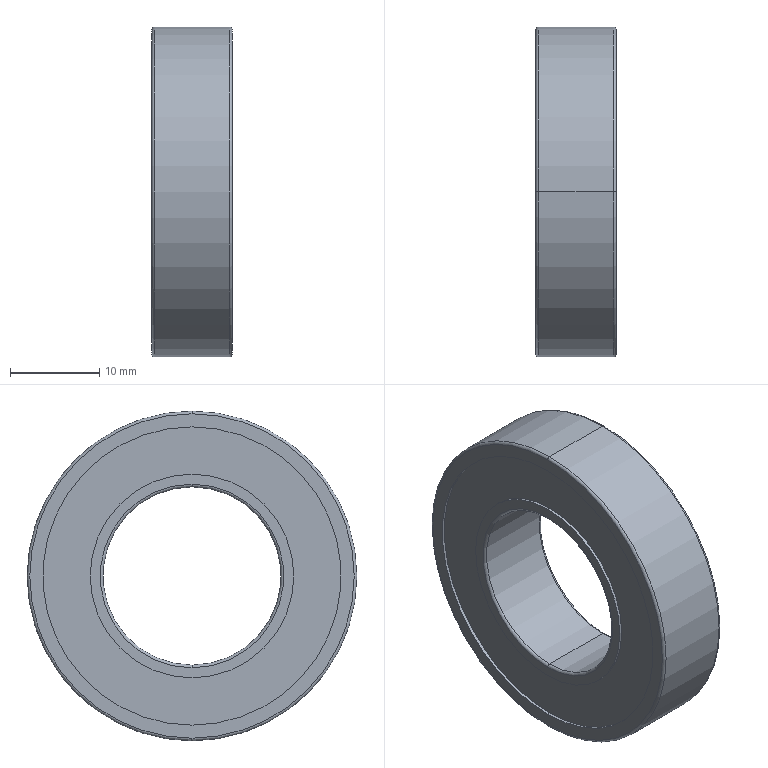Part | NX | features BREP 1 | 1 solid | 26 faces | box 9 x 37 x 37 mm | volume 6541 mm3 | cylinder 12 | torus 8 | plane 6 | commonest cylinder face diameters 22.858 x4 33.465 x4 20 x2 37 x2
STEP:
#1=CARTESIAN_POINT('',(8.7,0.,18.5));
#2=VERTEX_POINT('',#1);
#3=CARTESIAN_POINT('',(8.7,0.,-18.5));
#4=VERTEX_POINT('',#3);
#5=CARTESIAN_POINT('',(8.7,0.,0.));
#6=DIRECTION('',(-1.,0.,0.));
#7=DIRECTION('',(0.,0.,1.));
#8=AXIS2_PLACEMENT_3D('',#5,#6,#7);
#9=CIRCLE('',#8,18.5);
#10=EDGE_CURVE('',#2,#4,#9,.T.);
#11=ORIENTED_EDGE('',*,*,#10,.T.);
#12=CARTESIAN_POINT('',(0.3,0.,-18.5));
#13=VERTEX_POINT('',#12);
#14=CARTESIAN_POINT('',(9.,0.,-18.5));
#15=DIRECTION('',(-1.,0.,0.));
#16=VECTOR('',#15,1000.);
#17=LINE('',#14,#16);
#18=EDGE_CURVE('',#13,#4,#17,.F.);
#19=ORIENTED_EDGE('',*,*,#18,.F.);
#20=CARTESIAN_POINT('',(0.3,0.,18.5));
#21=VERTEX_POINT('',#20);
#22=CARTESIAN_POINT('',(0.3,0.,0.));
#23=DIRECTION('',(-1.,0.,0.));
#24=DIRECTION('',(0.,0.,1.));
#25=AXIS2_PLACEMENT_3D('',#22,#23,#24);
#26=CIRCLE('',#25,18.5);
#27=EDGE_CURVE('',#21,#13,#26,.T.);
#28=ORIENTED_EDGE('',*,*,#27,.F.);
#29=CARTESIAN_POINT('',(9.,0.,18.5));
#30=DIRECTION('',(-1.,0.,0.));
#31=VECTOR('',#30,1000.);
#32=LINE('',#29,#31);
#33=EDGE_CURVE('',#21,#2,#32,.F.);
#34=ORIENTED_EDGE('',*,*,#33,.T.);
#35=EDGE_LOOP('',(#11,#19,#28,#34));
#36=FACE_BOUND('',#35,.T.);
#37=CARTESIAN_POINT('',(9.,0.,0.));
#38=DIRECTION('',(-1.,0.,0.));
#39=DIRECTION('',(0.,0.,1.));
#40=AXIS2_PLACEMENT_3D('',#37,#38,#39);
#41=CYLINDRICAL_SURFACE('',#40,18.5);
#42=ADVANCED_FACE('',(#36),#41,.T.);
#43=CARTESIAN_POINT('',(9.,0.,18.2));
#44=VERTEX_POINT('',#43);
#45=CARTESIAN_POINT('',(9.,0.,-18.2));
#46=VERTEX_POINT('',#45);
#47=CARTESIAN_POINT('',(9.,0.,0.));
#48=DIRECTION('',(-1.,0.,0.));
#49=DIRECTION('',(0.,0.,1.));
#50=AXIS2_PLACEMENT_3D('',#47,#48,#49);
#51=CIRCLE('',#50,18.2);
#52=EDGE_CURVE('',#44,#46,#51,.T.);
#53=ORIENTED_EDGE('',*,*,#52,.T.);
#54=CARTESIAN_POINT('',(8.7,0.,-18.2));
#55=DIRECTION('',(0.,1.,0.));
#56=DIRECTION('',(0.,0.,1.));
#57=AXIS2_PLACEMENT_3D('',#54,#55,#56);
#58=CIRCLE('',#57,0.3);
#59=EDGE_CURVE('',#4,#46,#58,.F.);
#60=ORIENTED_EDGE('',*,*,#59,.F.);
#61=ORIENTED_EDGE('',*,*,#10,.F.);
#62=CARTESIAN_POINT('',(8.7,0.,18.2));
#63=DIRECTION('',(0.,-1.,0.));
#64=DIRECTION('',(0.,0.,-1.));
#65=AXIS2_PLACEMENT_3D('',#62,#63,#64);
#66=CIRCLE('',#65,0.3);
#67=EDGE_CURVE('',#2,#44,#66,.F.);
#68=ORIENTED_EDGE('',*,*,#67,.T.);
#69=EDGE_LOOP('',(#53,#60,#61,#68));
#70=FACE_BOUND('',#69,.T.);
#71=CARTESIAN_POINT('',(8.7,0.,0.));
#72=DIRECTION('',(-1.,0.,0.));
#73=DIRECTION('',(0.,0.,1.));
#74=AXIS2_PLACEMENT_3D('',#71,#72,#73);
#75=TOROIDAL_SURFACE('',#74,18.2,0.3);
#76=ADVANCED_FACE('',(#70),#75,.T.);
#77=CARTESIAN_POINT('',(9.,0.,-16.732));
#78=VERTEX_POINT('',#77);
#79=CARTESIAN_POINT('',(9.,0.,16.732));
#80=VERTEX_POINT('',#79);
#81=CARTESIAN_POINT('',(9.,0.,0.));
#82=DIRECTION('',(-1.,0.,0.));
#83=DIRECTION('',(0.,0.,1.));
#84=AXIS2_PLACEMENT_3D('',#81,#82,#83);
#85=CIRCLE('',#84,16.732);
#86=EDGE_CURVE('',#78,#80,#85,.T.);
#87=ORIENTED_EDGE('',*,*,#86,.F.);
#88=CARTESIAN_POINT('',(8.679,0.,-16.732));
#89=VERTEX_POINT('',#88);
#90=CARTESIAN_POINT('',(9.,0.,-16.732));
#91=DIRECTION('',(-1.,0.,0.));
#92=VECTOR('',#91,1000.);
#93=LINE('',#90,#92);
#94=EDGE_CURVE('',#89,#78,#93,.F.);
#95=ORIENTED_EDGE('',*,*,#94,.F.);
#96=CARTESIAN_POINT('',(8.679,0.,16.732));
#97=VERTEX_POINT('',#96);
#98=CARTESIAN_POINT('',(8.679,0.,0.));
#99=DIRECTION('',(-1.,0.,0.));
#100=DIRECTION('',(0.,0.,1.));
#101=AXIS2_PLACEMENT_3D('',#98,#99,#100);
#102=CIRCLE('',#101,16.732);
#103=EDGE_CURVE('',#89,#97,#102,.T.);
#104=ORIENTED_EDGE('',*,*,#103,.T.);
#105=CARTESIAN_POINT('',(9.,0.,16.732));
#106=DIRECTION('',(-1.,0.,0.));
#107=VECTOR('',#106,1000.);
#108=LINE('',#105,#107);
#109=EDGE_CURVE('',#97,#80,#108,.F.);
#110=ORIENTED_EDGE('',*,*,#109,.T.);
#111=EDGE_LOOP('',(#87,#95,#104,#110));
#112=FACE_BOUND('',#111,.T.);
#113=CARTESIAN_POINT('',(9.,0.,0.));
#114=DIRECTION('',(-1.,0.,0.));
#115=DIRECTION('',(0.,0.,1.));
#116=AXIS2_PLACEMENT_3D('',#113,#114,#115);
#117=CYLINDRICAL_SURFACE('',#116,16.732);
#118=ADVANCED_FACE('',(#112),#117,.F.);
#119=CARTESIAN_POINT('',(9.,0.,11.429));
#120=VERTEX_POINT('',#119);
#121=CARTESIAN_POINT('',(9.,0.,-11.429));
#122=VERTEX_POINT('',#121);
#123=CARTESIAN_POINT('',(9.,0.,0.));
#124=DIRECTION('',(-1.,0.,0.));
#125=DIRECTION('',(0.,0.,1.));
#126=AXIS2_PLACEMENT_3D('',#123,#124,#125);
#127=CIRCLE('',#126,11.429);
#128=EDGE_CURVE('',#120,#122,#127,.T.);
#129=ORIENTED_EDGE('',*,*,#128,.T.);
#130=CARTESIAN_POINT('',(8.679,0.,-11.429));
#131=VERTEX_POINT('',#130);
#132=CARTESIAN_POINT('',(9.,0.,-11.429));
#133=DIRECTION('',(-1.,0.,0.));
#134=VECTOR('',#133,1000.);
#135=LINE('',#132,#134);
#136=EDGE_CURVE('',#131,#122,#135,.F.);
#137=ORIENTED_EDGE('',*,*,#136,.F.);
#138=CARTESIAN_POINT('',(8.679,0.,11.429));
#139=VERTEX_POINT('',#138);
#140=CARTESIAN_POINT('',(8.679,0.,0.));
#141=DIRECTION('',(-1.,0.,0.));
#142=DIRECTION('',(0.,0.,1.));
#143=AXIS2_PLACEMENT_3D('',#140,#141,#142);
#144=CIRCLE('',#143,11.429);
#145=EDGE_CURVE('',#139,#131,#144,.T.);
#146=ORIENTED_EDGE('',*,*,#145,.F.);
#147=CARTESIAN_POINT('',(9.,0.,11.429));
#148=DIRECTION('',(-1.,0.,0.));
#149=VECTOR('',#148,1000.);
#150=LINE('',#147,#149);
#151=EDGE_CURVE('',#139,#120,#150,.F.);
#152=ORIENTED_EDGE('',*,*,#151,.T.);
#153=EDGE_LOOP('',(#129,#137,#146,#152));
#154=FACE_BOUND('',#153,.T.);
#155=CARTESIAN_POINT('',(9.,0.,0.));
#156=DIRECTION('',(-1.,0.,0.));
#157=DIRECTION('',(0.,0.,1.));
#158=AXIS2_PLACEMENT_3D('',#155,#156,#157);
#159=CYLINDRICAL_SURFACE('',#158,11.429);
#160=ADVANCED_FACE('',(#154),#159,.T.);
#161=CARTESIAN_POINT('',(8.7,0.,10.));
#162=VERTEX_POINT('',#161);
#163=CARTESIAN_POINT('',(8.7,0.,-10.));
#164=VERTEX_POINT('',#163);
#165=CARTESIAN_POINT('',(8.7,0.,0.));
#166=DIRECTION('',(-1.,0.,0.));
#167=DIRECTION('',(0.,0.,1.));
#168=AXIS2_PLACEMENT_3D('',#165,#166,#167);
#169=CIRCLE('',#168,10.);
#170=EDGE_CURVE('',#162,#164,#169,.T.);
#171=ORIENTED_EDGE('',*,*,#170,.T.);
#172=CARTESIAN_POINT('',(9.,0.,-10.3));
#173=VERTEX_POINT('',#172);
#174=CARTESIAN_POINT('',(8.7,0.,-10.3));
#175=DIRECTION('',(0.,1.,0.));
#176=DIRECTION('',(0.,0.,1.));
#177=AXIS2_PLACEMENT_3D('',#174,#175,#176);
#178=CIRCLE('',#177,0.3);
#179=EDGE_CURVE('',#173,#164,#178,.F.);
#180=ORIENTED_EDGE('',*,*,#179,.F.);
#181=CARTESIAN_POINT('',(9.,0.,10.3));
#182=VERTEX_POINT('',#181);
#183=CARTESIAN_POINT('',(9.,0.,0.));
#184=DIRECTION('',(-1.,0.,0.));
#185=DIRECTION('',(0.,0.,1.));
#186=AXIS2_PLACEMENT_3D('',#183,#184,#185);
#187=CIRCLE('',#186,10.3);
#188=EDGE_CURVE('',#182,#173,#187,.T.);
#189=ORIENTED_EDGE('',*,*,#188,.F.);
#190=CARTESIAN_POINT('',(8.7,0.,10.3));
#191=DIRECTION('',(0.,-1.,0.));
#192=DIRECTION('',(0.,0.,-1.));
#193=AXIS2_PLACEMENT_3D('',#190,#191,#192);
#194=CIRCLE('',#193,0.3);
#195=EDGE_CURVE('',#182,#162,#194,.F.);
#196=ORIENTED_EDGE('',*,*,#195,.T.);
#197=EDGE_LOOP('',(#171,#180,#189,#196));
#198=FACE_BOUND('',#197,.T.);
#199=CARTESIAN_POINT('',(8.7,0.,0.));
#200=DIRECTION('',(-1.,0.,0.));
#201=DIRECTION('',(0.,0.,1.));
#202=AXIS2_PLACEMENT_3D('',#199,#200,#201);
#203=TOROIDAL_SURFACE('',#202,10.3,0.3);
#204=ADVANCED_FACE('',(#198),#203,.T.);
#205=CARTESIAN_POINT('',(8.7,0.,0.));
#206=DIRECTION('',(-1.,0.,0.));
#207=DIRECTION('',(0.,0.,1.));
#208=AXIS2_PLACEMENT_3D('',#205,#206,#207);
#209=CIRCLE('',#208,10.);
#210=EDGE_CURVE('',#164,#162,#209,.T.);
#211=ORIENTED_EDGE('',*,*,#210,.F.);
#212=CARTESIAN_POINT('',(0.3,0.,-10.));
#213=VERTEX_POINT('',#212);
#214=CARTESIAN_POINT('',(9.,0.,-10.));
#215=DIRECTION('',(-1.,0.,0.));
#216=VECTOR('',#215,1000.);
#217=LINE('',#214,#216);
#218=EDGE_CURVE('',#213,#164,#217,.F.);
#219=ORIENTED_EDGE('',*,*,#218,.F.);
#220=CARTESIAN_POINT('',(0.3,0.,10.));
#221=VERTEX_POINT('',#220);
#222=CARTESIAN_POINT('',(0.3,0.,0.));
#223=DIRECTION('',(-1.,0.,0.));
#224=DIRECTION('',(0.,0.,1.));
#225=AXIS2_PLACEMENT_3D('',#222,#223,#224);
#226=CIRCLE('',#225,10.);
#227=EDGE_CURVE('',#213,#221,#226,.T.);
#228=ORIENTED_EDGE('',*,*,#227,.T.);
#229=CARTESIAN_POINT('',(9.,0.,10.));
#230=DIRECTION('',(-1.,0.,0.));
#231=VECTOR('',#230,1000.);
#232=LINE('',#229,#231);
#233=EDGE_CURVE('',#221,#162,#232,.F.);
#234=ORIENTED_EDGE('',*,*,#233,.T.);
#235=EDGE_LOOP('',(#211,#219,#228,#234));
#236=FACE_BOUND('',#235,.T.);
#237=CARTESIAN_POINT('',(9.,0.,0.));
#238=DIRECTION('',(-1.,0.,0.));
#239=DIRECTION('',(0.,0.,1.));
#240=AXIS2_PLACEMENT_3D('',#237,#238,#239);
#241=CYLINDRICAL_SURFACE('',#240,10.);
#242=ADVANCED_FACE('',(#236),#241,.F.);
#243=CARTESIAN_POINT('',(0.,0.,10.3));
#244=VERTEX_POINT('',#243);
#245=CARTESIAN_POINT('',(0.,0.,-10.3));
#246=VERTEX_POINT('',#245);
#247=CARTESIAN_POINT('',(0.,0.,0.));
#248=DIRECTION('',(-1.,0.,0.));
#249=DIRECTION('',(0.,0.,1.));
#250=AXIS2_PLACEMENT_3D('',#247,#248,#249);
#251=CIRCLE('',#250,10.3);
#252=EDGE_CURVE('',#244,#246,#251,.T.);
#253=ORIENTED_EDGE('',*,*,#252,.T.);
#254=CARTESIAN_POINT('',(0.3,0.,-10.3));
#255=DIRECTION('',(0.,1.,0.));
#256=DIRECTION('',(0.,0.,1.));
#257=AXIS2_PLACEMENT_3D('',#254,#255,#256);
#258=CIRCLE('',#257,0.3);
#259=EDGE_CURVE('',#213,#246,#258,.F.);
#260=ORIENTED_EDGE('',*,*,#259,.F.);
#261=CARTESIAN_POINT('',(0.3,0.,0.));
#262=DIRECTION('',(-1.,0.,0.));
#263=DIRECTION('',(0.,0.,1.));
#264=AXIS2_PLACEMENT_3D('',#261,#262,#263);
#265=CIRCLE('',#264,10.);
#266=EDGE_CURVE('',#221,#213,#265,.T.);
#267=ORIENTED_EDGE('',*,*,#266,.F.);
#268=CARTESIAN_POINT('',(0.3,0.,10.3));
#269=DIRECTION('',(0.,-1.,0.));
#270=DIRECTION('',(0.,0.,-1.));
#271=AXIS2_PLACEMENT_3D('',#268,#269,#270);
#272=CIRCLE('',#271,0.3);
#273=EDGE_CURVE('',#221,#244,#272,.F.);
#274=ORIENTED_EDGE('',*,*,#273,.T.);
#275=EDGE_LOOP('',(#253,#260,#267,#274));
#276=FACE_BOUND('',#275,.T.);
#277=CARTESIAN_POINT('',(0.3,0.,0.));
#278=DIRECTION('',(-1.,0.,0.));
#279=DIRECTION('',(0.,0.,1.));
#280=AXIS2_PLACEMENT_3D('',#277,#278,#279);
#281=TOROIDAL_SURFACE('',#280,10.3,0.3);
#282=ADVANCED_FACE('',(#276),#281,.T.);
#283=CARTESIAN_POINT('',(0.3212,0.,11.429));
#284=VERTEX_POINT('',#283);
#285=CARTESIAN_POINT('',(0.3212,0.,-11.429));
#286=VERTEX_POINT('',#285);
#287=CARTESIAN_POINT('',(0.3212,0.,0.));
#288=DIRECTION('',(-1.,0.,0.));
#289=DIRECTION('',(0.,0.,1.));
#290=AXIS2_PLACEMENT_3D('',#287,#288,#289);
#291=CIRCLE('',#290,11.429);
#292=EDGE_CURVE('',#284,#286,#291,.T.);
#293=ORIENTED_EDGE('',*,*,#292,.T.);
#294=CARTESIAN_POINT('',(0.,0.,-11.429));
#295=VERTEX_POINT('',#294);
#296=CARTESIAN_POINT('',(9.,0.,-11.429));
#297=DIRECTION('',(-1.,0.,0.));
#298=VECTOR('',#297,1000.);
#299=LINE('',#296,#298);
#300=EDGE_CURVE('',#295,#286,#299,.F.);
#301=ORIENTED_EDGE('',*,*,#300,.F.);
#302=CARTESIAN_POINT('',(0.,0.,11.429));
#303=VERTEX_POINT('',#302);
#304=CARTESIAN_POINT('',(0.,0.,0.));
#305=DIRECTION('',(-1.,0.,0.));
#306=DIRECTION('',(0.,0.,1.));
#307=AXIS2_PLACEMENT_3D('',#304,#305,#306);
#308=CIRCLE('',#307,11.429);
#309=EDGE_CURVE('',#303,#295,#308,.T.);
#310=ORIENTED_EDGE('',*,*,#309,.F.);
#311=CARTESIAN_POINT('',(9.,0.,11.429));
#312=DIRECTION('',(-1.,0.,0.));
#313=VECTOR('',#312,1000.);
#314=LINE('',#311,#313);
#315=EDGE_CURVE('',#303,#284,#314,.F.);
#316=ORIENTED_EDGE('',*,*,#315,.T.);
#317=EDGE_LOOP('',(#293,#301,#310,#316));
#318=FACE_BOUND('',#317,.T.);
#319=CARTESIAN_POINT('',(9.,0.,0.));
#320=DIRECTION('',(-1.,0.,0.));
#321=DIRECTION('',(0.,0.,1.));
#322=AXIS2_PLACEMENT_3D('',#319,#320,#321);
#323=CYLINDRICAL_SURFACE('',#322,11.429);
#324=ADVANCED_FACE('',(#318),#323,.T.);
#325=CARTESIAN_POINT('',(0.3212,0.,-16.732));
#326=VERTEX_POINT('',#325);
#327=CARTESIAN_POINT('',(0.3212,0.,16.732));
#328=VERTEX_POINT('',#327);
#329=CARTESIAN_POINT('',(0.3212,0.,0.));
#330=DIRECTION('',(-1.,0.,0.));
#331=DIRECTION('',(0.,0.,1.));
#332=AXIS2_PLACEMENT_3D('',#329,#330,#331);
#333=CIRCLE('',#332,16.732);
#334=EDGE_CURVE('',#326,#328,#333,.T.);
#335=ORIENTED_EDGE('',*,*,#334,.F.);
#336=CARTESIAN_POINT('',(0.,0.,-16.732));
#337=VERTEX_POINT('',#336);
#338=CARTESIAN_POINT('',(9.,0.,-16.732));
#339=DIRECTION('',(-1.,0.,0.));
#340=VECTOR('',#339,1000.);
#341=LINE('',#338,#340);
#342=EDGE_CURVE('',#337,#326,#341,.F.);
#343=ORIENTED_EDGE('',*,*,#342,.F.);
#344=CARTESIAN_POINT('',(0.,0.,16.732));
#345=VERTEX_POINT('',#344);
#346=CARTESIAN_POINT('',(0.,0.,0.));
#347=DIRECTION('',(-1.,0.,0.));
#348=DIRECTION('',(0.,0.,1.));
#349=AXIS2_PLACEMENT_3D('',#346,#347,#348);
#350=CIRCLE('',#349,16.732);
#351=EDGE_CURVE('',#337,#345,#350,.T.);
#352=ORIENTED_EDGE('',*,*,#351,.T.);
#353=CARTESIAN_POINT('',(9.,0.,16.732));
#354=DIRECTION('',(-1.,0.,0.));
#355=VECTOR('',#354,1000.);
#356=LINE('',#353,#355);
#357=EDGE_CURVE('',#345,#328,#356,.F.);
#358=ORIENTED_EDGE('',*,*,#357,.T.);
#359=EDGE_LOOP('',(#335,#343,#352,#358));
#360=FACE_BOUND('',#359,.T.);
#361=CARTESIAN_POINT('',(9.,0.,0.));
#362=DIRECTION('',(-1.,0.,0.));
#363=DIRECTION('',(0.,0.,1.));
#364=AXIS2_PLACEMENT_3D('',#361,#362,#363);
#365=CYLINDRICAL_SURFACE('',#364,16.732);
#366=ADVANCED_FACE('',(#360),#365,.F.);
#367=ORIENTED_EDGE('',*,*,#27,.T.);
#368=CARTESIAN_POINT('',(0.,0.,-18.2));
#369=VERTEX_POINT('',#368);
#370=CARTESIAN_POINT('',(0.3,0.,-18.2));
#371=DIRECTION('',(0.,1.,0.));
#372=DIRECTION('',(0.,0.,1.));
#373=AXIS2_PLACEMENT_3D('',#370,#371,#372);
#374=CIRCLE('',#373,0.3);
#375=EDGE_CURVE('',#369,#13,#374,.F.);
#376=ORIENTED_EDGE('',*,*,#375,.F.);
#377=CARTESIAN_POINT('',(0.,0.,18.2));
#378=VERTEX_POINT('',#377);
#379=CARTESIAN_POINT('',(0.,0.,0.));
#380=DIRECTION('',(-1.,0.,0.));
#381=DIRECTION('',(0.,0.,1.));
#382=AXIS2_PLACEMENT_3D('',#379,#380,#381);
#383=CIRCLE('',#382,18.2);
#384=EDGE_CURVE('',#378,#369,#383,.T.);
#385=ORIENTED_EDGE('',*,*,#384,.F.);
#386=CARTESIAN_POINT('',(0.3,0.,18.2));
#387=DIRECTION('',(0.,-1.,0.));
#388=DIRECTION('',(0.,0.,-1.));
#389=AXIS2_PLACEMENT_3D('',#386,#387,#388);
#390=CIRCLE('',#389,0.3);
#391=EDGE_CURVE('',#378,#21,#390,.F.);
#392=ORIENTED_EDGE('',*,*,#391,.T.);
#393=EDGE_LOOP('',(#367,#376,#385,#392));
#394=FACE_BOUND('',#393,.T.);
#395=CARTESIAN_POINT('',(0.3,0.,0.));
#396=DIRECTION('',(-1.,0.,0.));
#397=DIRECTION('',(0.,0.,1.));
#398=AXIS2_PLACEMENT_3D('',#395,#396,#397);
#399=TOROIDAL_SURFACE('',#398,18.2,0.3);
#400=ADVANCED_FACE('',(#394),#399,.T.);
#401=ORIENTED_EDGE('',*,*,#375,.T.);
#402=CARTESIAN_POINT('',(0.3,0.,0.));
#403=DIRECTION('',(-1.,0.,0.));
#404=DIRECTION('',(0.,0.,1.));
#405=AXIS2_PLACEMENT_3D('',#402,#403,#404);
#406=CIRCLE('',#405,18.5);
#407=EDGE_CURVE('',#13,#21,#406,.T.);
#408=ORIENTED_EDGE('',*,*,#407,.T.);
#409=ORIENTED_EDGE('',*,*,#391,.F.);
#410=CARTESIAN_POINT('',(0.,0.,0.));
#411=DIRECTION('',(-1.,0.,0.));
#412=DIRECTION('',(0.,0.,1.));
#413=AXIS2_PLACEMENT_3D('',#410,#411,#412);
#414=CIRCLE('',#413,18.2);
#415=EDGE_CURVE('',#369,#378,#414,.T.);
#416=ORIENTED_EDGE('',*,*,#415,.F.);
#417=EDGE_LOOP('',(#401,#408,#409,#416));
#418=FACE_BOUND('',#417,.T.);
#419=CARTESIAN_POINT('',(0.3,0.,0.));
#420=DIRECTION('',(-1.,0.,0.));
#421=DIRECTION('',(0.,0.,1.));
#422=AXIS2_PLACEMENT_3D('',#419,#420,#421);
#423=TOROIDAL_SURFACE('',#422,18.2,0.3);
#424=ADVANCED_FACE('',(#418),#423,.T.);
#425=ORIENTED_EDGE('',*,*,#384,.T.);
#426=ORIENTED_EDGE('',*,*,#415,.T.);
#427=EDGE_LOOP('',(#425,#426));
#428=FACE_BOUND('',#427,.T.);
#429=CARTESIAN_POINT('',(0.,0.,0.));
#430=DIRECTION('',(-1.,0.,0.));
#431=DIRECTION('',(0.,0.,1.));
#432=AXIS2_PLACEMENT_3D('',#429,#430,#431);
#433=CIRCLE('',#432,16.732);
#434=EDGE_CURVE('',#345,#337,#433,.T.);
#435=ORIENTED_EDGE('',*,*,#434,.F.);
#436=ORIENTED_EDGE('',*,*,#351,.F.);
#437=EDGE_LOOP('',(#435,#436));
#438=FACE_BOUND('',#437,.T.);
#439=CARTESIAN_POINT('',(0.,18.2,0.));
#440=DIRECTION('',(1.,0.,0.));
#441=DIRECTION('',(0.,1.,0.));
#442=AXIS2_PLACEMENT_3D('',#439,#440,#441);
#443=PLANE('',#442);
#444=ADVANCED_FACE('',(#428,#438),#443,.F.);
#445=ORIENTED_EDGE('',*,*,#342,.T.);
#446=CARTESIAN_POINT('',(0.3212,0.,0.));
#447=DIRECTION('',(-1.,0.,0.));
#448=DIRECTION('',(0.,0.,1.));
#449=AXIS2_PLACEMENT_3D('',#446,#447,#448);
#450=CIRCLE('',#449,16.732);
#451=EDGE_CURVE('',#328,#326,#450,.T.);
#452=ORIENTED_EDGE('',*,*,#451,.F.);
#453=ORIENTED_EDGE('',*,*,#357,.F.);
#454=ORIENTED_EDGE('',*,*,#434,.T.);
#455=EDGE_LOOP('',(#445,#452,#453,#454));
#456=FACE_BOUND('',#455,.T.);
#457=CARTESIAN_POINT('',(9.,0.,0.));
#458=DIRECTION('',(-1.,0.,0.));
#459=DIRECTION('',(0.,0.,1.));
#460=AXIS2_PLACEMENT_3D('',#457,#458,#459);
#461=CYLINDRICAL_SURFACE('',#460,16.732);
#462=ADVANCED_FACE('',(#456),#461,.F.);
#463=ORIENTED_EDGE('',*,*,#451,.T.);
#464=ORIENTED_EDGE('',*,*,#334,.T.);
#465=EDGE_LOOP('',(#463,#464));
#466=FACE_BOUND('',#465,.T.);
#467=ORIENTED_EDGE('',*,*,#292,.F.);
#468=CARTESIAN_POINT('',(0.3212,0.,0.));
#469=DIRECTION('',(-1.,0.,0.));
#470=DIRECTION('',(0.,0.,1.));
#471=AXIS2_PLACEMENT_3D('',#468,#469,#470);
#472=CIRCLE('',#471,11.429);
#473=EDGE_CURVE('',#286,#284,#472,.T.);
#474=ORIENTED_EDGE('',*,*,#473,.F.);
#475=EDGE_LOOP('',(#467,#474));
#476=FACE_BOUND('',#475,.T.);
#477=CARTESIAN_POINT('',(0.3212,16.732,0.));
#478=DIRECTION('',(1.,0.,0.));
#479=DIRECTION('',(0.,1.,0.));
#480=AXIS2_PLACEMENT_3D('',#477,#478,#479);
#481=PLANE('',#480);
#482=ADVANCED_FACE('',(#466,#476),#481,.F.);
#483=ORIENTED_EDGE('',*,*,#300,.T.);
#484=ORIENTED_EDGE('',*,*,#473,.T.);
#485=ORIENTED_EDGE('',*,*,#315,.F.);
#486=CARTESIAN_POINT('',(0.,0.,0.));
#487=DIRECTION('',(-1.,0.,0.));
#488=DIRECTION('',(0.,0.,1.));
#489=AXIS2_PLACEMENT_3D('',#486,#487,#488);
#490=CIRCLE('',#489,11.429);
#491=EDGE_CURVE('',#295,#303,#490,.T.);
#492=ORIENTED_EDGE('',*,*,#491,.F.);
#493=EDGE_LOOP('',(#483,#484,#485,#492));
#494=FACE_BOUND('',#493,.T.);
#495=CARTESIAN_POINT('',(9.,0.,0.));
#496=DIRECTION('',(-1.,0.,0.));
#497=DIRECTION('',(0.,0.,1.));
#498=AXIS2_PLACEMENT_3D('',#495,#496,#497);
#499=CYLINDRICAL_SURFACE('',#498,11.429);
#500=ADVANCED_FACE('',(#494),#499,.T.);
#501=ORIENTED_EDGE('',*,*,#309,.T.);
#502=ORIENTED_EDGE('',*,*,#491,.T.);
#503=EDGE_LOOP('',(#501,#502));
#504=FACE_BOUND('',#503,.T.);
#505=ORIENTED_EDGE('',*,*,#252,.F.);
#506=CARTESIAN_POINT('',(0.,0.,0.));
#507=DIRECTION('',(-1.,0.,0.));
#508=DIRECTION('',(0.,0.,1.));
#509=AXIS2_PLACEMENT_3D('',#506,#507,#508);
#510=CIRCLE('',#509,10.3);
#511=EDGE_CURVE('',#246,#244,#510,.T.);
#512=ORIENTED_EDGE('',*,*,#511,.F.);
#513=EDGE_LOOP('',(#505,#512));
#514=FACE_BOUND('',#513,.T.);
#515=CARTESIAN_POINT('',(0.,11.429,0.));
#516=DIRECTION('',(1.,0.,0.));
#517=DIRECTION('',(0.,1.,0.));
#518=AXIS2_PLACEMENT_3D('',#515,#516,#517);
#519=PLANE('',#518);
#520=ADVANCED_FACE('',(#504,#514),#519,.F.);
#521=ORIENTED_EDGE('',*,*,#259,.T.);
#522=ORIENTED_EDGE('',*,*,#511,.T.);
#523=ORIENTED_EDGE('',*,*,#273,.F.);
#524=ORIENTED_EDGE('',*,*,#227,.F.);
#525=EDGE_LOOP('',(#521,#522,#523,#524));
#526=FACE_BOUND('',#525,.T.);
#527=CARTESIAN_POINT('',(0.3,0.,0.));
#528=DIRECTION('',(-1.,0.,0.));
#529=DIRECTION('',(0.,0.,1.));
#530=AXIS2_PLACEMENT_3D('',#527,#528,#529);
#531=TOROIDAL_SURFACE('',#530,10.3,0.3);
#532=ADVANCED_FACE('',(#526),#531,.T.);
#533=ORIENTED_EDGE('',*,*,#218,.T.);
#534=ORIENTED_EDGE('',*,*,#170,.F.);
#535=ORIENTED_EDGE('',*,*,#233,.F.);
#536=ORIENTED_EDGE('',*,*,#266,.T.);
#537=EDGE_LOOP('',(#533,#534,#535,#536));
#538=FACE_BOUND('',#537,.T.);
#539=CARTESIAN_POINT('',(9.,0.,0.));
#540=DIRECTION('',(-1.,0.,0.));
#541=DIRECTION('',(0.,0.,1.));
#542=AXIS2_PLACEMENT_3D('',#539,#540,#541);
#543=CYLINDRICAL_SURFACE('',#542,10.);
#544=ADVANCED_FACE('',(#538),#543,.F.);
#545=ORIENTED_EDGE('',*,*,#179,.T.);
#546=ORIENTED_EDGE('',*,*,#210,.T.);
#547=ORIENTED_EDGE('',*,*,#195,.F.);
#548=CARTESIAN_POINT('',(9.,0.,0.));
#549=DIRECTION('',(-1.,0.,0.));
#550=DIRECTION('',(0.,0.,1.));
#551=AXIS2_PLACEMENT_3D('',#548,#549,#550);
#552=CIRCLE('',#551,10.3);
#553=EDGE_CURVE('',#173,#182,#552,.T.);
#554=ORIENTED_EDGE('',*,*,#553,.F.);
#555=EDGE_LOOP('',(#545,#546,#547,#554));
#556=FACE_BOUND('',#555,.T.);
#557=CARTESIAN_POINT('',(8.7,0.,0.));
#558=DIRECTION('',(-1.,0.,0.));
#559=DIRECTION('',(0.,0.,1.));
#560=AXIS2_PLACEMENT_3D('',#557,#558,#559);
#561=TOROIDAL_SURFACE('',#560,10.3,0.3);
#562=ADVANCED_FACE('',(#556),#561,.T.);
#563=ORIENTED_EDGE('',*,*,#128,.F.);
#564=CARTESIAN_POINT('',(9.,0.,0.));
#565=DIRECTION('',(-1.,0.,0.));
#566=DIRECTION('',(0.,0.,1.));
#567=AXIS2_PLACEMENT_3D('',#564,#565,#566);
#568=CIRCLE('',#567,11.429);
#569=EDGE_CURVE('',#122,#120,#568,.T.);
#570=ORIENTED_EDGE('',*,*,#569,.F.);
#571=EDGE_LOOP('',(#563,#570));
#572=FACE_BOUND('',#571,.T.);
#573=ORIENTED_EDGE('',*,*,#188,.T.);
#574=ORIENTED_EDGE('',*,*,#553,.T.);
#575=EDGE_LOOP('',(#573,#574));
#576=FACE_BOUND('',#575,.T.);
#577=CARTESIAN_POINT('',(9.,10.3,0.));
#578=DIRECTION('',(-1.,0.,0.));
#579=DIRECTION('',(0.,0.,1.));
#580=AXIS2_PLACEMENT_3D('',#577,#578,#579);
#581=PLANE('',#580);
#582=ADVANCED_FACE('',(#572,#576),#581,.F.);
#583=ORIENTED_EDGE('',*,*,#136,.T.);
#584=ORIENTED_EDGE('',*,*,#569,.T.);
#585=ORIENTED_EDGE('',*,*,#151,.F.);
#586=CARTESIAN_POINT('',(8.679,0.,0.));
#587=DIRECTION('',(-1.,0.,0.));
#588=DIRECTION('',(0.,0.,1.));
#589=AXIS2_PLACEMENT_3D('',#586,#587,#588);
#590=CIRCLE('',#589,11.429);
#591=EDGE_CURVE('',#131,#139,#590,.T.);
#592=ORIENTED_EDGE('',*,*,#591,.F.);
#593=EDGE_LOOP('',(#583,#584,#585,#592));
#594=FACE_BOUND('',#593,.T.);
#595=CARTESIAN_POINT('',(9.,0.,0.));
#596=DIRECTION('',(-1.,0.,0.));
#597=DIRECTION('',(0.,0.,1.));
#598=AXIS2_PLACEMENT_3D('',#595,#596,#597);
#599=CYLINDRICAL_SURFACE('',#598,11.429);
#600=ADVANCED_FACE('',(#594),#599,.T.);
#601=CARTESIAN_POINT('',(8.679,0.,0.));
#602=DIRECTION('',(-1.,0.,0.));
#603=DIRECTION('',(0.,0.,1.));
#604=AXIS2_PLACEMENT_3D('',#601,#602,#603);
#605=CIRCLE('',#604,16.732);
#606=EDGE_CURVE('',#97,#89,#605,.T.);
#607=ORIENTED_EDGE('',*,*,#606,.F.);
#608=ORIENTED_EDGE('',*,*,#103,.F.);
#609=EDGE_LOOP('',(#607,#608));
#610=FACE_BOUND('',#609,.T.);
#611=ORIENTED_EDGE('',*,*,#145,.T.);
#612=ORIENTED_EDGE('',*,*,#591,.T.);
#613=EDGE_LOOP('',(#611,#612));
#614=FACE_BOUND('',#613,.T.);
#615=CARTESIAN_POINT('',(8.679,11.429,0.));
#616=DIRECTION('',(-1.,0.,0.));
#617=DIRECTION('',(0.,0.,1.));
#618=AXIS2_PLACEMENT_3D('',#615,#616,#617);
#619=PLANE('',#618);
#620=ADVANCED_FACE('',(#610,#614),#619,.F.);
#621=ORIENTED_EDGE('',*,*,#94,.T.);
#622=CARTESIAN_POINT('',(9.,0.,0.));
#623=DIRECTION('',(-1.,0.,0.));
#624=DIRECTION('',(0.,0.,1.));
#625=AXIS2_PLACEMENT_3D('',#622,#623,#624);
#626=CIRCLE('',#625,16.732);
#627=EDGE_CURVE('',#80,#78,#626,.T.);
#628=ORIENTED_EDGE('',*,*,#627,.F.);
#629=ORIENTED_EDGE('',*,*,#109,.F.);
#630=ORIENTED_EDGE('',*,*,#606,.T.);
#631=EDGE_LOOP('',(#621,#628,#629,#630));
#632=FACE_BOUND('',#631,.T.);
#633=CARTESIAN_POINT('',(9.,0.,0.));
#634=DIRECTION('',(-1.,0.,0.));
#635=DIRECTION('',(0.,0.,1.));
#636=AXIS2_PLACEMENT_3D('',#633,#634,#635);
#637=CYLINDRICAL_SURFACE('',#636,16.732);
#638=ADVANCED_FACE('',(#632),#637,.F.);
#639=ORIENTED_EDGE('',*,*,#52,.F.);
#640=CARTESIAN_POINT('',(9.,0.,0.));
#641=DIRECTION('',(-1.,0.,0.));
#642=DIRECTION('',(0.,0.,1.));
#643=AXIS2_PLACEMENT_3D('',#640,#641,#642);
#644=CIRCLE('',#643,18.2);
#645=EDGE_CURVE('',#46,#44,#644,.T.);
#646=ORIENTED_EDGE('',*,*,#645,.F.);
#647=EDGE_LOOP('',(#639,#646));
#648=FACE_BOUND('',#647,.T.);
#649=ORIENTED_EDGE('',*,*,#627,.T.);
#650=ORIENTED_EDGE('',*,*,#86,.T.);
#651=EDGE_LOOP('',(#649,#650));
#652=FACE_BOUND('',#651,.T.);
#653=CARTESIAN_POINT('',(9.,16.732,0.));
#654=DIRECTION('',(-1.,0.,0.));
#655=DIRECTION('',(0.,0.,1.));
#656=AXIS2_PLACEMENT_3D('',#653,#654,#655);
#657=PLANE('',#656);
#658=ADVANCED_FACE('',(#648,#652),#657,.F.);
#659=ORIENTED_EDGE('',*,*,#59,.T.);
#660=ORIENTED_EDGE('',*,*,#645,.T.);
#661=ORIENTED_EDGE('',*,*,#67,.F.);
#662=CARTESIAN_POINT('',(8.7,0.,0.));
#663=DIRECTION('',(-1.,0.,0.));
#664=DIRECTION('',(0.,0.,1.));
#665=AXIS2_PLACEMENT_3D('',#662,#663,#664);
#666=CIRCLE('',#665,18.5);
#667=EDGE_CURVE('',#4,#2,#666,.T.);
#668=ORIENTED_EDGE('',*,*,#667,.F.);
#669=EDGE_LOOP('',(#659,#660,#661,#668));
#670=FACE_BOUND('',#669,.T.);
#671=CARTESIAN_POINT('',(8.7,0.,0.));
#672=DIRECTION('',(-1.,0.,0.));
#673=DIRECTION('',(0.,0.,1.));
#674=AXIS2_PLACEMENT_3D('',#671,#672,#673);
#675=TOROIDAL_SURFACE('',#674,18.2,0.3);
#676=ADVANCED_FACE('',(#670),#675,.T.);
#677=ORIENTED_EDGE('',*,*,#18,.T.);
#678=ORIENTED_EDGE('',*,*,#667,.T.);
#679=ORIENTED_EDGE('',*,*,#33,.F.);
#680=ORIENTED_EDGE('',*,*,#407,.F.);
#681=EDGE_LOOP('',(#677,#678,#679,#680));
#682=FACE_BOUND('',#681,.T.);
#683=CARTESIAN_POINT('',(9.,0.,0.));
#684=DIRECTION('',(-1.,0.,0.));
#685=DIRECTION('',(0.,0.,1.));
#686=AXIS2_PLACEMENT_3D('',#683,#684,#685);
#687=CYLINDRICAL_SURFACE('',#686,18.5);
#688=ADVANCED_FACE('',(#682),#687,.T.);
#689=CLOSED_SHELL('',(#42,#76,#118,#160,#204,#242,#282,#324,#366,#400,#424,#444,#462,#482,#500,#520,#532,#544,#562,#582,#600,#620,#638,#658,#676,#688));
#690=MANIFOLD_SOLID_BREP('',#689);
#691=(LENGTH_UNIT()NAMED_UNIT(*)SI_UNIT(.MILLI.,.METRE.));
#692=UNCERTAINTY_MEASURE_WITH_UNIT(LENGTH_MEASURE(0.00001),#691,'','');
#693=(NAMED_UNIT(*)PLANE_ANGLE_UNIT()SI_UNIT($,.RADIAN.));
#694=(NAMED_UNIT(*)SI_UNIT($,.STERADIAN.)SOLID_ANGLE_UNIT());
#695=(GEOMETRIC_REPRESENTATION_CONTEXT(3)GLOBAL_UNCERTAINTY_ASSIGNED_CONTEXT((#692))GLOBAL_UNIT_ASSIGNED_CONTEXT((#691,#693,#694))REPRESENTATION_CONTEXT('',''));
#696=ADVANCED_BREP_SHAPE_REPRESENTATION('',(#690),#695);